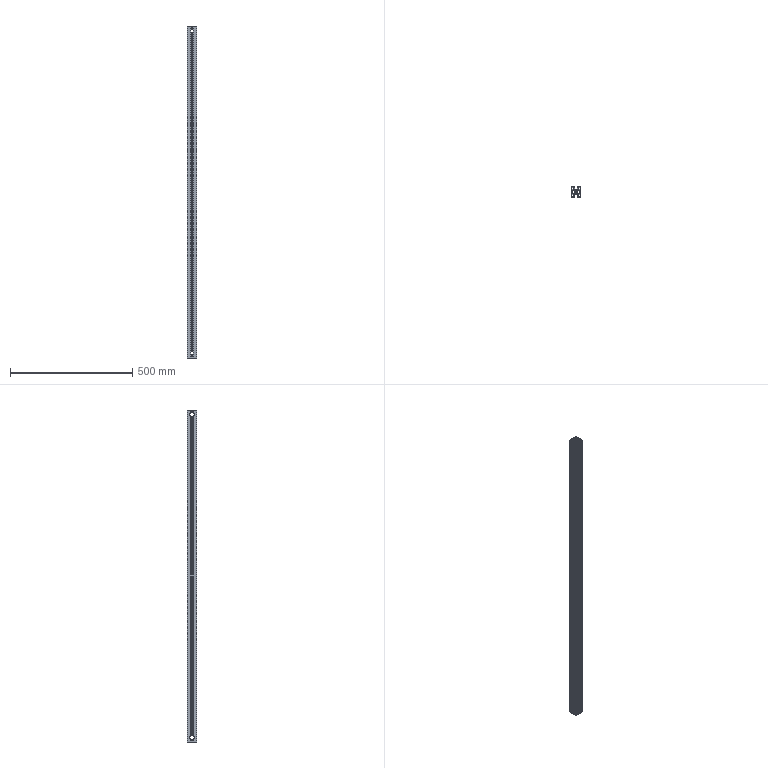Part | SolidWorks | features BaseBody 1, HoleWzd 1, MoveFace 1 | 1 solid | 345 faces | box 40 x 40 x 1360 mm | volume 721762 mm3 | plane 250 | cylinder 95 | commonest cylinder face diameters 0.6 x24 10 x24 2 x16 6.8 x15 19 x12 3 x4